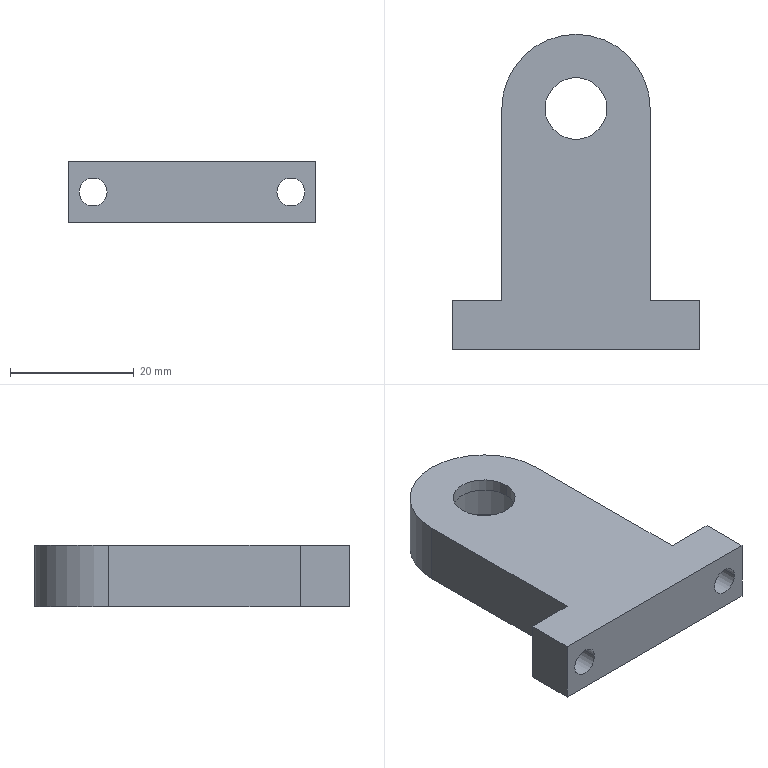Part | Creo | features CURVE 4, CUT 3, DATUM PLANE 3, COORDINATE SYSTEM 1, PROTRUSION 1 | 1 solid | 22 faces | box 40 x 51 x 10 mm | volume 10314 mm3 | plane 11 | cylinder 11 | commonest cylinder face diameters 4.5 x4 10 x2 15.636 x2 19 x2 24 x1
STEP:
#1=CARTESIAN_POINT('',(0.,0.,0.));
#2=DIRECTION('',(0.,0.,1.));
#3=DIRECTION('',(1.,0.,0.));
#4=AXIS2_PLACEMENT_3D('',#1,#2,#3);
#5=CARTESIAN_POINT('',(12.,39.,0.));
#6=VERTEX_POINT('',#5);
#7=CARTESIAN_POINT('',(-12.,39.,0.));
#8=VERTEX_POINT('',#7);
#9=CARTESIAN_POINT('',(0.,39.,0.));
#10=DIRECTION('',(0.,0.,1.));
#11=DIRECTION('',(1.,0.,0.));
#12=AXIS2_PLACEMENT_3D('',#9,#10,#11);
#13=CIRCLE('',#12,12.);
#14=EDGE_CURVE('',#6,#8,#13,.T.);
#15=ORIENTED_EDGE('',*,*,#14,.T.);
#16=CARTESIAN_POINT('',(-12.,8.,0.));
#17=VERTEX_POINT('',#16);
#18=CARTESIAN_POINT('',(-12.,39.,0.));
#19=DIRECTION('',(0.,-1.,0.));
#20=VECTOR('',#19,31.);
#21=LINE('',#18,#20);
#22=EDGE_CURVE('',#8,#17,#21,.T.);
#23=ORIENTED_EDGE('',*,*,#22,.T.);
#24=CARTESIAN_POINT('',(-20.,8.,0.));
#25=VERTEX_POINT('',#24);
#26=CARTESIAN_POINT('',(-12.,8.,0.));
#27=DIRECTION('',(-1.,0.,0.));
#28=VECTOR('',#27,8.);
#29=LINE('',#26,#28);
#30=EDGE_CURVE('',#17,#25,#29,.T.);
#31=ORIENTED_EDGE('',*,*,#30,.T.);
#32=CARTESIAN_POINT('',(-20.,0.,0.));
#33=VERTEX_POINT('',#32);
#34=CARTESIAN_POINT('',(-20.,8.,0.));
#35=DIRECTION('',(0.,-1.,0.));
#36=VECTOR('',#35,8.);
#37=LINE('',#34,#36);
#38=EDGE_CURVE('',#25,#33,#37,.T.);
#39=ORIENTED_EDGE('',*,*,#38,.T.);
#40=CARTESIAN_POINT('',(20.,0.,0.));
#41=VERTEX_POINT('',#40);
#42=CARTESIAN_POINT('',(-20.,0.,0.));
#43=DIRECTION('',(1.,0.,0.));
#44=VECTOR('',#43,40.);
#45=LINE('',#42,#44);
#46=EDGE_CURVE('',#33,#41,#45,.T.);
#47=ORIENTED_EDGE('',*,*,#46,.T.);
#48=CARTESIAN_POINT('',(20.,8.,0.));
#49=VERTEX_POINT('',#48);
#50=CARTESIAN_POINT('',(20.,0.,0.));
#51=DIRECTION('',(0.,1.,0.));
#52=VECTOR('',#51,8.);
#53=LINE('',#50,#52);
#54=EDGE_CURVE('',#41,#49,#53,.T.);
#55=ORIENTED_EDGE('',*,*,#54,.T.);
#56=CARTESIAN_POINT('',(12.,8.,0.));
#57=VERTEX_POINT('',#56);
#58=CARTESIAN_POINT('',(20.,8.,0.));
#59=DIRECTION('',(-1.,0.,0.));
#60=VECTOR('',#59,8.);
#61=LINE('',#58,#60);
#62=EDGE_CURVE('',#49,#57,#61,.T.);
#63=ORIENTED_EDGE('',*,*,#62,.T.);
#64=CARTESIAN_POINT('',(12.,8.,0.));
#65=DIRECTION('',(0.,1.,0.));
#66=VECTOR('',#65,31.);
#67=LINE('',#64,#66);
#68=EDGE_CURVE('',#57,#6,#67,.T.);
#69=ORIENTED_EDGE('',*,*,#68,.T.);
#70=EDGE_LOOP('',(#15,#23,#31,#39,#47,#55,#63,#69));
#71=FACE_OUTER_BOUND('',#70,.F.);
#72=CARTESIAN_POINT('',(-9.5,39.,0.));
#73=VERTEX_POINT('',#72);
#74=CARTESIAN_POINT('',(9.5,39.,0.));
#75=VERTEX_POINT('',#74);
#76=CARTESIAN_POINT('',(0.,39.,0.));
#77=DIRECTION('',(0.,0.,-1.));
#78=DIRECTION('',(-1.,0.,0.));
#79=AXIS2_PLACEMENT_3D('',#76,#77,#78);
#80=CIRCLE('',#79,9.5);
#81=EDGE_CURVE('',#73,#75,#80,.T.);
#82=ORIENTED_EDGE('',*,*,#81,.T.);
#83=CARTESIAN_POINT('',(0.,39.,0.));
#84=DIRECTION('',(0.,0.,-1.));
#85=DIRECTION('',(1.,0.,0.));
#86=AXIS2_PLACEMENT_3D('',#83,#84,#85);
#87=CIRCLE('',#86,9.5);
#88=EDGE_CURVE('',#75,#73,#87,.T.);
#89=ORIENTED_EDGE('',*,*,#88,.T.);
#90=EDGE_LOOP('',(#82,#89));
#91=FACE_BOUND('',#90,.F.);
#92=CARTESIAN_POINT('',(0.,0.,0.));
#93=DIRECTION('',(0.,0.,1.));
#94=DIRECTION('',(1.,0.,0.));
#95=AXIS2_PLACEMENT_3D('',#92,#93,#94);
#96=PLANE('',#95);
#97=ADVANCED_FACE('',(#71,#91),#96,.F.);
#98=ORIENTED_EDGE('',*,*,#14,.F.);
#99=CARTESIAN_POINT('',(12.,39.,10.));
#100=VERTEX_POINT('',#99);
#101=CARTESIAN_POINT('',(12.,39.,0.));
#102=DIRECTION('',(0.,0.,1.));
#103=VECTOR('',#102,10.);
#104=LINE('',#101,#103);
#105=EDGE_CURVE('',#6,#100,#104,.T.);
#106=ORIENTED_EDGE('',*,*,#105,.T.);
#107=CARTESIAN_POINT('',(-12.,39.,10.));
#108=VERTEX_POINT('',#107);
#109=CARTESIAN_POINT('',(0.,39.,10.));
#110=DIRECTION('',(0.,0.,1.));
#111=DIRECTION('',(1.,0.,0.));
#112=AXIS2_PLACEMENT_3D('',#109,#110,#111);
#113=CIRCLE('',#112,12.);
#114=EDGE_CURVE('',#100,#108,#113,.T.);
#115=ORIENTED_EDGE('',*,*,#114,.T.);
#116=CARTESIAN_POINT('',(-12.,39.,0.));
#117=DIRECTION('',(0.,0.,1.));
#118=VECTOR('',#117,10.);
#119=LINE('',#116,#118);
#120=EDGE_CURVE('',#8,#108,#119,.T.);
#121=ORIENTED_EDGE('',*,*,#120,.F.);
#122=EDGE_LOOP('',(#98,#106,#115,#121));
#123=FACE_OUTER_BOUND('',#122,.F.);
#124=CARTESIAN_POINT('',(0.,39.,0.));
#125=DIRECTION('',(0.,0.,1.));
#126=DIRECTION('',(1.,0.,0.));
#127=AXIS2_PLACEMENT_3D('',#124,#125,#126);
#128=CYLINDRICAL_SURFACE('',#127,12.);
#129=ADVANCED_FACE('',(#123),#128,.T.);
#130=ORIENTED_EDGE('',*,*,#68,.F.);
#131=CARTESIAN_POINT('',(12.,8.,10.));
#132=VERTEX_POINT('',#131);
#133=CARTESIAN_POINT('',(12.,8.,0.));
#134=DIRECTION('',(0.,0.,1.));
#135=VECTOR('',#134,10.);
#136=LINE('',#133,#135);
#137=EDGE_CURVE('',#57,#132,#136,.T.);
#138=ORIENTED_EDGE('',*,*,#137,.T.);
#139=CARTESIAN_POINT('',(12.,8.,10.));
#140=DIRECTION('',(0.,1.,0.));
#141=VECTOR('',#140,31.);
#142=LINE('',#139,#141);
#143=EDGE_CURVE('',#132,#100,#142,.T.);
#144=ORIENTED_EDGE('',*,*,#143,.T.);
#145=ORIENTED_EDGE('',*,*,#105,.F.);
#146=EDGE_LOOP('',(#130,#138,#144,#145));
#147=FACE_OUTER_BOUND('',#146,.F.);
#148=CARTESIAN_POINT('',(12.,8.,0.));
#149=DIRECTION('',(1.,0.,0.));
#150=DIRECTION('',(0.,1.,0.));
#151=AXIS2_PLACEMENT_3D('',#148,#149,#150);
#152=PLANE('',#151);
#153=ADVANCED_FACE('',(#147),#152,.T.);
#154=ORIENTED_EDGE('',*,*,#62,.F.);
#155=CARTESIAN_POINT('',(20.,8.,10.));
#156=VERTEX_POINT('',#155);
#157=CARTESIAN_POINT('',(20.,8.,0.));
#158=DIRECTION('',(0.,0.,1.));
#159=VECTOR('',#158,10.);
#160=LINE('',#157,#159);
#161=EDGE_CURVE('',#49,#156,#160,.T.);
#162=ORIENTED_EDGE('',*,*,#161,.T.);
#163=CARTESIAN_POINT('',(20.,8.,10.));
#164=DIRECTION('',(-1.,0.,0.));
#165=VECTOR('',#164,8.);
#166=LINE('',#163,#165);
#167=EDGE_CURVE('',#156,#132,#166,.T.);
#168=ORIENTED_EDGE('',*,*,#167,.T.);
#169=ORIENTED_EDGE('',*,*,#137,.F.);
#170=EDGE_LOOP('',(#154,#162,#168,#169));
#171=FACE_OUTER_BOUND('',#170,.F.);
#172=CARTESIAN_POINT('',(18.25,8.,5.));
#173=VERTEX_POINT('',#172);
#174=CARTESIAN_POINT('',(13.75,8.,5.));
#175=VERTEX_POINT('',#174);
#176=CARTESIAN_POINT('',(16.,8.,5.));
#177=DIRECTION('',(0.,1.,0.));
#178=DIRECTION('',(1.,0.,0.));
#179=AXIS2_PLACEMENT_3D('',#176,#177,#178);
#180=CIRCLE('',#179,2.25);
#181=EDGE_CURVE('',#173,#175,#180,.T.);
#182=ORIENTED_EDGE('',*,*,#181,.T.);
#183=CARTESIAN_POINT('',(16.,8.,5.));
#184=DIRECTION('',(0.,1.,0.));
#185=DIRECTION('',(-1.,0.,0.));
#186=AXIS2_PLACEMENT_3D('',#183,#184,#185);
#187=CIRCLE('',#186,2.25);
#188=EDGE_CURVE('',#175,#173,#187,.T.);
#189=ORIENTED_EDGE('',*,*,#188,.T.);
#190=EDGE_LOOP('',(#182,#189));
#191=FACE_BOUND('',#190,.F.);
#192=CARTESIAN_POINT('',(20.,8.,0.));
#193=DIRECTION('',(0.,1.,0.));
#194=DIRECTION('',(-1.,0.,0.));
#195=AXIS2_PLACEMENT_3D('',#192,#193,#194);
#196=PLANE('',#195);
#197=ADVANCED_FACE('',(#171,#191),#196,.T.);
#198=ORIENTED_EDGE('',*,*,#54,.F.);
#199=CARTESIAN_POINT('',(20.,0.,10.));
#200=VERTEX_POINT('',#199);
#201=CARTESIAN_POINT('',(20.,0.,0.));
#202=DIRECTION('',(0.,0.,1.));
#203=VECTOR('',#202,10.);
#204=LINE('',#201,#203);
#205=EDGE_CURVE('',#41,#200,#204,.T.);
#206=ORIENTED_EDGE('',*,*,#205,.T.);
#207=CARTESIAN_POINT('',(20.,0.,10.));
#208=DIRECTION('',(0.,1.,0.));
#209=VECTOR('',#208,8.);
#210=LINE('',#207,#209);
#211=EDGE_CURVE('',#200,#156,#210,.T.);
#212=ORIENTED_EDGE('',*,*,#211,.T.);
#213=ORIENTED_EDGE('',*,*,#161,.F.);
#214=EDGE_LOOP('',(#198,#206,#212,#213));
#215=FACE_OUTER_BOUND('',#214,.F.);
#216=CARTESIAN_POINT('',(20.,0.,0.));
#217=DIRECTION('',(1.,0.,0.));
#218=DIRECTION('',(0.,1.,0.));
#219=AXIS2_PLACEMENT_3D('',#216,#217,#218);
#220=PLANE('',#219);
#221=ADVANCED_FACE('',(#215),#220,.T.);
#222=ORIENTED_EDGE('',*,*,#46,.F.);
#223=CARTESIAN_POINT('',(-20.,0.,10.));
#224=VERTEX_POINT('',#223);
#225=CARTESIAN_POINT('',(-20.,0.,0.));
#226=DIRECTION('',(0.,0.,1.));
#227=VECTOR('',#226,10.);
#228=LINE('',#225,#227);
#229=EDGE_CURVE('',#33,#224,#228,.T.);
#230=ORIENTED_EDGE('',*,*,#229,.T.);
#231=CARTESIAN_POINT('',(-20.,0.,10.));
#232=DIRECTION('',(1.,0.,0.));
#233=VECTOR('',#232,40.);
#234=LINE('',#231,#233);
#235=EDGE_CURVE('',#224,#200,#234,.T.);
#236=ORIENTED_EDGE('',*,*,#235,.T.);
#237=ORIENTED_EDGE('',*,*,#205,.F.);
#238=EDGE_LOOP('',(#222,#230,#236,#237));
#239=FACE_OUTER_BOUND('',#238,.F.);
#240=CARTESIAN_POINT('',(18.25,0.,5.));
#241=VERTEX_POINT('',#240);
#242=CARTESIAN_POINT('',(13.75,0.,5.));
#243=VERTEX_POINT('',#242);
#244=CARTESIAN_POINT('',(16.,0.,5.));
#245=DIRECTION('',(0.,1.,0.));
#246=DIRECTION('',(1.,0.,0.));
#247=AXIS2_PLACEMENT_3D('',#244,#245,#246);
#248=CIRCLE('',#247,2.25);
#249=EDGE_CURVE('',#241,#243,#248,.T.);
#250=ORIENTED_EDGE('',*,*,#249,.F.);
#251=CARTESIAN_POINT('',(16.,0.,5.));
#252=DIRECTION('',(0.,1.,0.));
#253=DIRECTION('',(-1.,0.,0.));
#254=AXIS2_PLACEMENT_3D('',#251,#252,#253);
#255=CIRCLE('',#254,2.25);
#256=EDGE_CURVE('',#243,#241,#255,.T.);
#257=ORIENTED_EDGE('',*,*,#256,.F.);
#258=EDGE_LOOP('',(#250,#257));
#259=FACE_BOUND('',#258,.F.);
#260=CARTESIAN_POINT('',(-13.75,0.,5.));
#261=VERTEX_POINT('',#260);
#262=CARTESIAN_POINT('',(-18.25,0.,5.));
#263=VERTEX_POINT('',#262);
#264=CARTESIAN_POINT('',(-16.,0.,5.));
#265=DIRECTION('',(0.,1.,0.));
#266=DIRECTION('',(1.,0.,0.));
#267=AXIS2_PLACEMENT_3D('',#264,#265,#266);
#268=CIRCLE('',#267,2.25);
#269=EDGE_CURVE('',#261,#263,#268,.T.);
#270=ORIENTED_EDGE('',*,*,#269,.F.);
#271=CARTESIAN_POINT('',(-16.,0.,5.));
#272=DIRECTION('',(0.,1.,0.));
#273=DIRECTION('',(-1.,0.,0.));
#274=AXIS2_PLACEMENT_3D('',#271,#272,#273);
#275=CIRCLE('',#274,2.25);
#276=EDGE_CURVE('',#263,#261,#275,.T.);
#277=ORIENTED_EDGE('',*,*,#276,.F.);
#278=EDGE_LOOP('',(#270,#277));
#279=FACE_BOUND('',#278,.F.);
#280=CARTESIAN_POINT('',(-20.,0.,0.));
#281=DIRECTION('',(0.,-1.,0.));
#282=DIRECTION('',(1.,0.,0.));
#283=AXIS2_PLACEMENT_3D('',#280,#281,#282);
#284=PLANE('',#283);
#285=ADVANCED_FACE('',(#239,#259,#279),#284,.T.);
#286=ORIENTED_EDGE('',*,*,#38,.F.);
#287=CARTESIAN_POINT('',(-20.,8.,10.));
#288=VERTEX_POINT('',#287);
#289=CARTESIAN_POINT('',(-20.,8.,0.));
#290=DIRECTION('',(0.,0.,1.));
#291=VECTOR('',#290,10.);
#292=LINE('',#289,#291);
#293=EDGE_CURVE('',#25,#288,#292,.T.);
#294=ORIENTED_EDGE('',*,*,#293,.T.);
#295=CARTESIAN_POINT('',(-20.,8.,10.));
#296=DIRECTION('',(0.,-1.,0.));
#297=VECTOR('',#296,8.);
#298=LINE('',#295,#297);
#299=EDGE_CURVE('',#288,#224,#298,.T.);
#300=ORIENTED_EDGE('',*,*,#299,.T.);
#301=ORIENTED_EDGE('',*,*,#229,.F.);
#302=EDGE_LOOP('',(#286,#294,#300,#301));
#303=FACE_OUTER_BOUND('',#302,.F.);
#304=CARTESIAN_POINT('',(-20.,8.,0.));
#305=DIRECTION('',(-1.,0.,0.));
#306=DIRECTION('',(0.,-1.,0.));
#307=AXIS2_PLACEMENT_3D('',#304,#305,#306);
#308=PLANE('',#307);
#309=ADVANCED_FACE('',(#303),#308,.T.);
#310=ORIENTED_EDGE('',*,*,#30,.F.);
#311=CARTESIAN_POINT('',(-12.,8.,10.));
#312=VERTEX_POINT('',#311);
#313=CARTESIAN_POINT('',(-12.,8.,0.));
#314=DIRECTION('',(0.,0.,1.));
#315=VECTOR('',#314,10.);
#316=LINE('',#313,#315);
#317=EDGE_CURVE('',#17,#312,#316,.T.);
#318=ORIENTED_EDGE('',*,*,#317,.T.);
#319=CARTESIAN_POINT('',(-12.,8.,10.));
#320=DIRECTION('',(-1.,0.,0.));
#321=VECTOR('',#320,8.);
#322=LINE('',#319,#321);
#323=EDGE_CURVE('',#312,#288,#322,.T.);
#324=ORIENTED_EDGE('',*,*,#323,.T.);
#325=ORIENTED_EDGE('',*,*,#293,.F.);
#326=EDGE_LOOP('',(#310,#318,#324,#325));
#327=FACE_OUTER_BOUND('',#326,.F.);
#328=CARTESIAN_POINT('',(-13.75,8.,5.));
#329=VERTEX_POINT('',#328);
#330=CARTESIAN_POINT('',(-18.25,8.,5.));
#331=VERTEX_POINT('',#330);
#332=CARTESIAN_POINT('',(-16.,8.,5.));
#333=DIRECTION('',(0.,1.,0.));
#334=DIRECTION('',(1.,0.,0.));
#335=AXIS2_PLACEMENT_3D('',#332,#333,#334);
#336=CIRCLE('',#335,2.25);
#337=EDGE_CURVE('',#329,#331,#336,.T.);
#338=ORIENTED_EDGE('',*,*,#337,.T.);
#339=CARTESIAN_POINT('',(-16.,8.,5.));
#340=DIRECTION('',(0.,1.,0.));
#341=DIRECTION('',(-1.,0.,0.));
#342=AXIS2_PLACEMENT_3D('',#339,#340,#341);
#343=CIRCLE('',#342,2.25);
#344=EDGE_CURVE('',#331,#329,#343,.T.);
#345=ORIENTED_EDGE('',*,*,#344,.T.);
#346=EDGE_LOOP('',(#338,#345));
#347=FACE_BOUND('',#346,.F.);
#348=CARTESIAN_POINT('',(-12.,8.,0.));
#349=DIRECTION('',(0.,1.,0.));
#350=DIRECTION('',(-1.,0.,0.));
#351=AXIS2_PLACEMENT_3D('',#348,#349,#350);
#352=PLANE('',#351);
#353=ADVANCED_FACE('',(#327,#347),#352,.T.);
#354=ORIENTED_EDGE('',*,*,#22,.F.);
#355=ORIENTED_EDGE('',*,*,#120,.T.);
#356=CARTESIAN_POINT('',(-12.,39.,10.));
#357=DIRECTION('',(0.,-1.,0.));
#358=VECTOR('',#357,31.);
#359=LINE('',#356,#358);
#360=EDGE_CURVE('',#108,#312,#359,.T.);
#361=ORIENTED_EDGE('',*,*,#360,.T.);
#362=ORIENTED_EDGE('',*,*,#317,.F.);
#363=EDGE_LOOP('',(#354,#355,#361,#362));
#364=FACE_OUTER_BOUND('',#363,.F.);
#365=CARTESIAN_POINT('',(-12.,39.,0.));
#366=DIRECTION('',(-1.,0.,0.));
#367=DIRECTION('',(0.,-1.,0.));
#368=AXIS2_PLACEMENT_3D('',#365,#366,#367);
#369=PLANE('',#368);
#370=ADVANCED_FACE('',(#364),#369,.T.);
#371=ORIENTED_EDGE('',*,*,#114,.F.);
#372=ORIENTED_EDGE('',*,*,#143,.F.);
#373=ORIENTED_EDGE('',*,*,#167,.F.);
#374=ORIENTED_EDGE('',*,*,#211,.F.);
#375=ORIENTED_EDGE('',*,*,#235,.F.);
#376=ORIENTED_EDGE('',*,*,#299,.F.);
#377=ORIENTED_EDGE('',*,*,#323,.F.);
#378=ORIENTED_EDGE('',*,*,#360,.F.);
#379=EDGE_LOOP('',(#371,#372,#373,#374,#375,#376,#377,#378));
#380=FACE_OUTER_BOUND('',#379,.F.);
#381=CARTESIAN_POINT('',(5.,39.,10.));
#382=VERTEX_POINT('',#381);
#383=CARTESIAN_POINT('',(-5.,39.,10.));
#384=VERTEX_POINT('',#383);
#385=CARTESIAN_POINT('',(0.,39.,10.));
#386=DIRECTION('',(0.,0.,-1.));
#387=DIRECTION('',(1.,0.,0.));
#388=AXIS2_PLACEMENT_3D('',#385,#386,#387);
#389=CIRCLE('',#388,5.);
#390=EDGE_CURVE('',#382,#384,#389,.T.);
#391=ORIENTED_EDGE('',*,*,#390,.F.);
#392=CARTESIAN_POINT('',(0.,39.,10.));
#393=DIRECTION('',(0.,0.,-1.));
#394=DIRECTION('',(-1.,0.,0.));
#395=AXIS2_PLACEMENT_3D('',#392,#393,#394);
#396=CIRCLE('',#395,5.);
#397=EDGE_CURVE('',#384,#382,#396,.T.);
#398=ORIENTED_EDGE('',*,*,#397,.F.);
#399=EDGE_LOOP('',(#391,#398));
#400=FACE_BOUND('',#399,.F.);
#401=CARTESIAN_POINT('',(0.,0.,10.));
#402=DIRECTION('',(0.,0.,1.));
#403=DIRECTION('',(1.,0.,0.));
#404=AXIS2_PLACEMENT_3D('',#401,#402,#403);
#405=PLANE('',#404);
#406=ADVANCED_FACE('',(#380,#400),#405,.T.);
#407=CARTESIAN_POINT('',(-5.,39.,8.));
#408=VERTEX_POINT('',#407);
#409=CARTESIAN_POINT('',(5.,39.,8.));
#410=VERTEX_POINT('',#409);
#411=CARTESIAN_POINT('',(0.,39.,8.));
#412=DIRECTION('',(0.,0.,1.));
#413=DIRECTION('',(-1.,0.,0.));
#414=AXIS2_PLACEMENT_3D('',#411,#412,#413);
#415=CIRCLE('',#414,5.);
#416=EDGE_CURVE('',#408,#410,#415,.T.);
#417=ORIENTED_EDGE('',*,*,#416,.T.);
#418=CARTESIAN_POINT('',(5.,39.,8.));
#419=DIRECTION('',(0.,0.,1.));
#420=VECTOR('',#419,2.);
#421=LINE('',#418,#420);
#422=EDGE_CURVE('',#410,#382,#421,.T.);
#423=ORIENTED_EDGE('',*,*,#422,.T.);
#424=ORIENTED_EDGE('',*,*,#390,.T.);
#425=CARTESIAN_POINT('',(-5.,39.,8.));
#426=DIRECTION('',(0.,0.,1.));
#427=VECTOR('',#426,2.);
#428=LINE('',#425,#427);
#429=EDGE_CURVE('',#408,#384,#428,.T.);
#430=ORIENTED_EDGE('',*,*,#429,.F.);
#431=EDGE_LOOP('',(#417,#423,#424,#430));
#432=FACE_OUTER_BOUND('',#431,.F.);
#433=CARTESIAN_POINT('',(0.,39.,0.));
#434=DIRECTION('',(0.,0.,1.));
#435=DIRECTION('',(1.,0.,0.));
#436=AXIS2_PLACEMENT_3D('',#433,#434,#435);
#437=CYLINDRICAL_SURFACE('',#436,5.);
#438=ADVANCED_FACE('',(#432),#437,.F.);
#439=CARTESIAN_POINT('',(-7.818,39.,8.));
#440=VERTEX_POINT('',#439);
#441=CARTESIAN_POINT('',(7.818,39.,8.));
#442=VERTEX_POINT('',#441);
#443=CARTESIAN_POINT('',(0.,39.,8.));
#444=DIRECTION('',(0.,0.,-1.));
#445=DIRECTION('',(-1.,0.,0.));
#446=AXIS2_PLACEMENT_3D('',#443,#444,#445);
#447=CIRCLE('',#446,7.818);
#448=EDGE_CURVE('',#440,#442,#447,.T.);
#449=ORIENTED_EDGE('',*,*,#448,.F.);
#450=CARTESIAN_POINT('',(0.,39.,8.));
#451=DIRECTION('',(0.,0.,-1.));
#452=DIRECTION('',(1.,0.,0.));
#453=AXIS2_PLACEMENT_3D('',#450,#451,#452);
#454=CIRCLE('',#453,7.818);
#455=EDGE_CURVE('',#442,#440,#454,.T.);
#456=ORIENTED_EDGE('',*,*,#455,.F.);
#457=EDGE_LOOP('',(#449,#456));
#458=FACE_OUTER_BOUND('',#457,.F.);
#459=ORIENTED_EDGE('',*,*,#416,.F.);
#460=CARTESIAN_POINT('',(0.,39.,8.));
#461=DIRECTION('',(0.,0.,1.));
#462=DIRECTION('',(1.,0.,0.));
#463=AXIS2_PLACEMENT_3D('',#460,#461,#462);
#464=CIRCLE('',#463,5.);
#465=EDGE_CURVE('',#410,#408,#464,.T.);
#466=ORIENTED_EDGE('',*,*,#465,.F.);
#467=EDGE_LOOP('',(#459,#466));
#468=FACE_BOUND('',#467,.F.);
#469=CARTESIAN_POINT('',(0.,0.,8.));
#470=DIRECTION('',(0.,0.,-1.));
#471=DIRECTION('',(-1.,0.,0.));
#472=AXIS2_PLACEMENT_3D('',#469,#470,#471);
#473=PLANE('',#472);
#474=ADVANCED_FACE('',(#458,#468),#473,.T.);
#475=CARTESIAN_POINT('',(-7.818,39.,7.));
#476=VERTEX_POINT('',#475);
#477=CARTESIAN_POINT('',(7.818,39.,7.));
#478=VERTEX_POINT('',#477);
#479=CARTESIAN_POINT('',(0.,39.,7.));
#480=DIRECTION('',(0.,0.,-1.));
#481=DIRECTION('',(-1.,0.,0.));
#482=AXIS2_PLACEMENT_3D('',#479,#480,#481);
#483=CIRCLE('',#482,7.818);
#484=EDGE_CURVE('',#476,#478,#483,.T.);
#485=ORIENTED_EDGE('',*,*,#484,.F.);
#486=CARTESIAN_POINT('',(-7.818,39.,7.));
#487=DIRECTION('',(0.,0.,1.));
#488=VECTOR('',#487,1.);
#489=LINE('',#486,#488);
#490=EDGE_CURVE('',#476,#440,#489,.T.);
#491=ORIENTED_EDGE('',*,*,#490,.T.);
#492=ORIENTED_EDGE('',*,*,#448,.T.);
#493=CARTESIAN_POINT('',(7.818,39.,7.));
#494=DIRECTION('',(0.,0.,1.));
#495=VECTOR('',#494,1.);
#496=LINE('',#493,#495);
#497=EDGE_CURVE('',#478,#442,#496,.T.);
#498=ORIENTED_EDGE('',*,*,#497,.F.);
#499=EDGE_LOOP('',(#485,#491,#492,#498));
#500=FACE_OUTER_BOUND('',#499,.F.);
#501=CARTESIAN_POINT('',(0.,39.,7.));
#502=DIRECTION('',(0.,0.,-1.));
#503=DIRECTION('',(-1.,0.,0.));
#504=AXIS2_PLACEMENT_3D('',#501,#502,#503);
#505=CYLINDRICAL_SURFACE('',#504,7.818);
#506=ADVANCED_FACE('',(#500),#505,.F.);
#507=CARTESIAN_POINT('',(-9.5,39.,7.));
#508=VERTEX_POINT('',#507);
#509=CARTESIAN_POINT('',(9.5,39.,7.));
#510=VERTEX_POINT('',#509);
#511=CARTESIAN_POINT('',(0.,39.,7.));
#512=DIRECTION('',(0.,0.,-1.));
#513=DIRECTION('',(-1.,0.,0.));
#514=AXIS2_PLACEMENT_3D('',#511,#512,#513);
#515=CIRCLE('',#514,9.5);
#516=EDGE_CURVE('',#508,#510,#515,.T.);
#517=ORIENTED_EDGE('',*,*,#516,.F.);
#518=CARTESIAN_POINT('',(0.,39.,7.));
#519=DIRECTION('',(0.,0.,-1.));
#520=DIRECTION('',(1.,0.,0.));
#521=AXIS2_PLACEMENT_3D('',#518,#519,#520);
#522=CIRCLE('',#521,9.5);
#523=EDGE_CURVE('',#510,#508,#522,.T.);
#524=ORIENTED_EDGE('',*,*,#523,.F.);
#525=EDGE_LOOP('',(#517,#524));
#526=FACE_OUTER_BOUND('',#525,.F.);
#527=ORIENTED_EDGE('',*,*,#484,.T.);
#528=CARTESIAN_POINT('',(0.,39.,7.));
#529=DIRECTION('',(0.,0.,-1.));
#530=DIRECTION('',(1.,0.,0.));
#531=AXIS2_PLACEMENT_3D('',#528,#529,#530);
#532=CIRCLE('',#531,7.818);
#533=EDGE_CURVE('',#478,#476,#532,.T.);
#534=ORIENTED_EDGE('',*,*,#533,.T.);
#535=EDGE_LOOP('',(#527,#534));
#536=FACE_BOUND('',#535,.F.);
#537=CARTESIAN_POINT('',(0.,0.,7.));
#538=DIRECTION('',(0.,0.,-1.));
#539=DIRECTION('',(-1.,0.,0.));
#540=AXIS2_PLACEMENT_3D('',#537,#538,#539);
#541=PLANE('',#540);
#542=ADVANCED_FACE('',(#526,#536),#541,.T.);
#543=ORIENTED_EDGE('',*,*,#81,.F.);
#544=CARTESIAN_POINT('',(-9.5,39.,0.));
#545=DIRECTION('',(0.,0.,1.));
#546=VECTOR('',#545,7.);
#547=LINE('',#544,#546);
#548=EDGE_CURVE('',#73,#508,#547,.T.);
#549=ORIENTED_EDGE('',*,*,#548,.T.);
#550=ORIENTED_EDGE('',*,*,#516,.T.);
#551=CARTESIAN_POINT('',(9.5,39.,0.));
#552=DIRECTION('',(0.,0.,1.));
#553=VECTOR('',#552,7.);
#554=LINE('',#551,#553);
#555=EDGE_CURVE('',#75,#510,#554,.T.);
#556=ORIENTED_EDGE('',*,*,#555,.F.);
#557=EDGE_LOOP('',(#543,#549,#550,#556));
#558=FACE_OUTER_BOUND('',#557,.F.);
#559=CARTESIAN_POINT('',(0.,39.,0.));
#560=DIRECTION('',(0.,0.,-1.));
#561=DIRECTION('',(-1.,0.,0.));
#562=AXIS2_PLACEMENT_3D('',#559,#560,#561);
#563=CYLINDRICAL_SURFACE('',#562,9.5);
#564=ADVANCED_FACE('',(#558),#563,.F.);
#565=ORIENTED_EDGE('',*,*,#88,.F.);
#566=ORIENTED_EDGE('',*,*,#555,.T.);
#567=ORIENTED_EDGE('',*,*,#523,.T.);
#568=ORIENTED_EDGE('',*,*,#548,.F.);
#569=EDGE_LOOP('',(#565,#566,#567,#568));
#570=FACE_OUTER_BOUND('',#569,.F.);
#571=CARTESIAN_POINT('',(0.,39.,0.));
#572=DIRECTION('',(0.,0.,-1.));
#573=DIRECTION('',(-1.,0.,0.));
#574=AXIS2_PLACEMENT_3D('',#571,#572,#573);
#575=CYLINDRICAL_SURFACE('',#574,9.5);
#576=ADVANCED_FACE('',(#570),#575,.F.);
#577=ORIENTED_EDGE('',*,*,#533,.F.);
#578=ORIENTED_EDGE('',*,*,#497,.T.);
#579=ORIENTED_EDGE('',*,*,#455,.T.);
#580=ORIENTED_EDGE('',*,*,#490,.F.);
#581=EDGE_LOOP('',(#577,#578,#579,#580));
#582=FACE_OUTER_BOUND('',#581,.F.);
#583=CARTESIAN_POINT('',(0.,39.,7.));
#584=DIRECTION('',(0.,0.,-1.));
#585=DIRECTION('',(-1.,0.,0.));
#586=AXIS2_PLACEMENT_3D('',#583,#584,#585);
#587=CYLINDRICAL_SURFACE('',#586,7.818);
#588=ADVANCED_FACE('',(#582),#587,.F.);
#589=ORIENTED_EDGE('',*,*,#465,.T.);
#590=ORIENTED_EDGE('',*,*,#429,.T.);
#591=ORIENTED_EDGE('',*,*,#397,.T.);
#592=ORIENTED_EDGE('',*,*,#422,.F.);
#593=EDGE_LOOP('',(#589,#590,#591,#592));
#594=FACE_OUTER_BOUND('',#593,.F.);
#595=CARTESIAN_POINT('',(0.,39.,0.));
#596=DIRECTION('',(0.,0.,1.));
#597=DIRECTION('',(1.,0.,0.));
#598=AXIS2_PLACEMENT_3D('',#595,#596,#597);
#599=CYLINDRICAL_SURFACE('',#598,5.);
#600=ADVANCED_FACE('',(#594),#599,.F.);
#601=ORIENTED_EDGE('',*,*,#337,.F.);
#602=CARTESIAN_POINT('',(-13.75,8.,5.));
#603=DIRECTION('',(0.,-1.,0.));
#604=VECTOR('',#603,8.);
#605=LINE('',#602,#604);
#606=EDGE_CURVE('',#329,#261,#605,.T.);
#607=ORIENTED_EDGE('',*,*,#606,.T.);
#608=ORIENTED_EDGE('',*,*,#269,.T.);
#609=CARTESIAN_POINT('',(-18.25,8.,5.));
#610=DIRECTION('',(0.,-1.,0.));
#611=VECTOR('',#610,8.);
#612=LINE('',#609,#611);
#613=EDGE_CURVE('',#331,#263,#612,.T.);
#614=ORIENTED_EDGE('',*,*,#613,.F.);
#615=EDGE_LOOP('',(#601,#607,#608,#614));
#616=FACE_OUTER_BOUND('',#615,.F.);
#617=CARTESIAN_POINT('',(-16.,8.,5.));
#618=DIRECTION('',(0.,1.,0.));
#619=DIRECTION('',(1.,0.,0.));
#620=AXIS2_PLACEMENT_3D('',#617,#618,#619);
#621=CYLINDRICAL_SURFACE('',#620,2.25);
#622=ADVANCED_FACE('',(#616),#621,.F.);
#623=ORIENTED_EDGE('',*,*,#344,.F.);
#624=ORIENTED_EDGE('',*,*,#613,.T.);
#625=ORIENTED_EDGE('',*,*,#276,.T.);
#626=ORIENTED_EDGE('',*,*,#606,.F.);
#627=EDGE_LOOP('',(#623,#624,#625,#626));
#628=FACE_OUTER_BOUND('',#627,.F.);
#629=CARTESIAN_POINT('',(-16.,8.,5.));
#630=DIRECTION('',(0.,1.,0.));
#631=DIRECTION('',(1.,0.,0.));
#632=AXIS2_PLACEMENT_3D('',#629,#630,#631);
#633=CYLINDRICAL_SURFACE('',#632,2.25);
#634=ADVANCED_FACE('',(#628),#633,.F.);
#635=ORIENTED_EDGE('',*,*,#249,.T.);
#636=CARTESIAN_POINT('',(13.75,8.,5.));
#637=DIRECTION('',(0.,-1.,0.));
#638=VECTOR('',#637,8.);
#639=LINE('',#636,#638);
#640=EDGE_CURVE('',#175,#243,#639,.T.);
#641=ORIENTED_EDGE('',*,*,#640,.F.);
#642=ORIENTED_EDGE('',*,*,#181,.F.);
#643=CARTESIAN_POINT('',(18.25,8.,5.));
#644=DIRECTION('',(0.,-1.,0.));
#645=VECTOR('',#644,8.);
#646=LINE('',#643,#645);
#647=EDGE_CURVE('',#173,#241,#646,.T.);
#648=ORIENTED_EDGE('',*,*,#647,.T.);
#649=EDGE_LOOP('',(#635,#641,#642,#648));
#650=FACE_OUTER_BOUND('',#649,.F.);
#651=CARTESIAN_POINT('',(16.,8.,5.));
#652=DIRECTION('',(0.,1.,0.));
#653=DIRECTION('',(1.,0.,0.));
#654=AXIS2_PLACEMENT_3D('',#651,#652,#653);
#655=CYLINDRICAL_SURFACE('',#654,2.25);
#656=ADVANCED_FACE('',(#650),#655,.F.);
#657=ORIENTED_EDGE('',*,*,#256,.T.);
#658=ORIENTED_EDGE('',*,*,#647,.F.);
#659=ORIENTED_EDGE('',*,*,#188,.F.);
#660=ORIENTED_EDGE('',*,*,#640,.T.);
#661=EDGE_LOOP('',(#657,#658,#659,#660));
#662=FACE_OUTER_BOUND('',#661,.F.);
#663=CARTESIAN_POINT('',(16.,8.,5.));
#664=DIRECTION('',(0.,1.,0.));
#665=DIRECTION('',(1.,0.,0.));
#666=AXIS2_PLACEMENT_3D('',#663,#664,#665);
#667=CYLINDRICAL_SURFACE('',#666,2.25);
#668=ADVANCED_FACE('',(#662),#667,.F.);
#669=CLOSED_SHELL('',(#97,#129,#153,#197,#221,#285,#309,#353,#370,#406,#438,#474,#506,#542,#564,#576,#588,#600,#622,#634,#656,#668));
#670=MANIFOLD_SOLID_BREP('',#669);
#671=(LENGTH_UNIT()NAMED_UNIT(*)SI_UNIT(.MILLI.,.METRE.));
#672=UNCERTAINTY_MEASURE_WITH_UNIT(LENGTH_MEASURE(0.006558),#671,'','');
#673=(NAMED_UNIT(*)PLANE_ANGLE_UNIT()SI_UNIT($,.RADIAN.));
#674=PLANE_ANGLE_MEASURE_WITH_UNIT(PLANE_ANGLE_MEASURE(0.01745),#673);
#675=(CONVERSION_BASED_UNIT('DEGREE',#674)NAMED_UNIT(*)PLANE_ANGLE_UNIT());
#676=(NAMED_UNIT(*)SI_UNIT($,.STERADIAN.)SOLID_ANGLE_UNIT());
#677=(GEOMETRIC_REPRESENTATION_CONTEXT(3)GLOBAL_UNCERTAINTY_ASSIGNED_CONTEXT((#672))GLOBAL_UNIT_ASSIGNED_CONTEXT((#671,#675,#676))REPRESENTATION_CONTEXT('',''));
#678=ADVANCED_BREP_SHAPE_REPRESENTATION('',(#4,#670),#677);